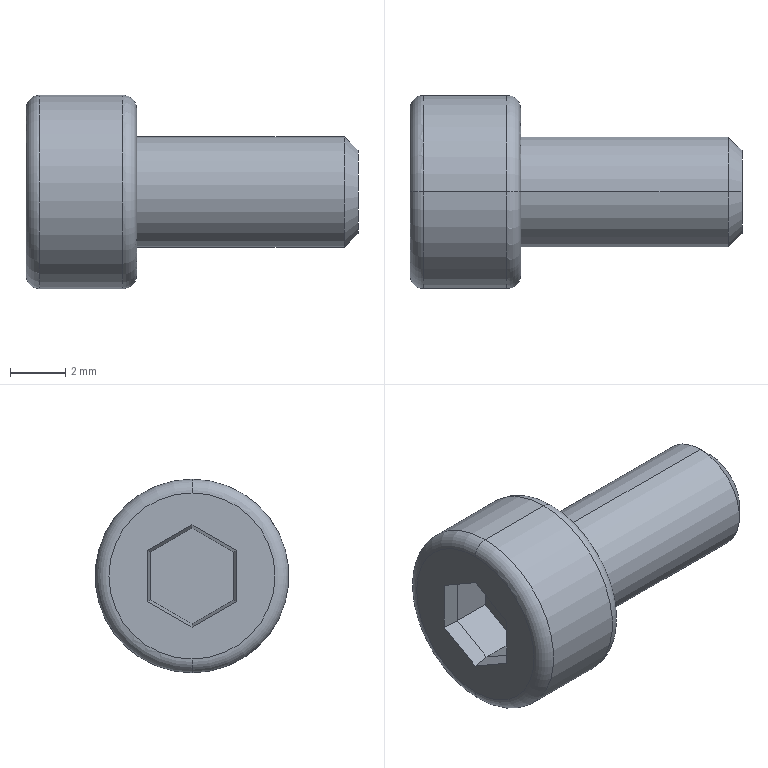Part | SolidWorks | features Chamfer 2, Fillet 1, ICE 1, Revolution 1 | 1 solid | 26 faces | box 12 x 7 x 7 mm | volume 234.855 mm3 | plane 16 | torus 4 | cylinder 4 | cone 2 | commonest cylinder face diameters 4 x2 7 x2
STEP:
#1=CARTESIAN_POINT('',(12.,0.,-1.5));
#2=VERTEX_POINT('',#1);
#3=CARTESIAN_POINT('',(12.,0.,1.5));
#4=VERTEX_POINT('',#3);
#5=CARTESIAN_POINT('',(12.,0.,0.));
#6=DIRECTION('',(1.,0.,0.));
#7=DIRECTION('',(0.,0.,1.));
#8=AXIS2_PLACEMENT_3D('',#5,#6,#7);
#9=CIRCLE('',#8,1.5);
#10=EDGE_CURVE('',#2,#4,#9,.T.);
#11=ORIENTED_EDGE('',*,*,#10,.F.);
#12=CARTESIAN_POINT('',(11.5,0.,-2.));
#13=VERTEX_POINT('',#12);
#14=CARTESIAN_POINT('',(11.5,0.,-2.));
#15=DIRECTION('',(-0.7071,0.,-0.7071));
#16=VECTOR('',#15,1000.);
#17=LINE('',#14,#16);
#18=EDGE_CURVE('',#2,#13,#17,.T.);
#19=ORIENTED_EDGE('',*,*,#18,.T.);
#20=CARTESIAN_POINT('',(11.5,0.,2.));
#21=VERTEX_POINT('',#20);
#22=CARTESIAN_POINT('',(11.5,0.,0.));
#23=DIRECTION('',(-1.,0.,0.));
#24=DIRECTION('',(0.,0.,1.));
#25=AXIS2_PLACEMENT_3D('',#22,#23,#24);
#26=CIRCLE('',#25,2.);
#27=EDGE_CURVE('',#21,#13,#26,.T.);
#28=ORIENTED_EDGE('',*,*,#27,.F.);
#29=CARTESIAN_POINT('',(11.5,0.,2.));
#30=DIRECTION('',(-0.7071,0.,0.7071));
#31=VECTOR('',#30,1000.);
#32=LINE('',#29,#31);
#33=EDGE_CURVE('',#4,#21,#32,.T.);
#34=ORIENTED_EDGE('',*,*,#33,.F.);
#35=EDGE_LOOP('',(#11,#19,#28,#34));
#36=FACE_OUTER_BOUND('',#35,.T.);
#37=CARTESIAN_POINT('',(11.5,0.,0.));
#38=DIRECTION('',(-1.,0.,0.));
#39=DIRECTION('',(0.,0.,1.));
#40=AXIS2_PLACEMENT_3D('',#37,#38,#39);
#41=CONICAL_SURFACE('',#40,2.,0.7854);
#42=ADVANCED_FACE('',(#36),#41,.T.);
#43=CARTESIAN_POINT('',(0.,0.,3.));
#44=VERTEX_POINT('',#43);
#45=CARTESIAN_POINT('',(0.,0.,-3.));
#46=VERTEX_POINT('',#45);
#47=CARTESIAN_POINT('',(0.,0.,0.));
#48=DIRECTION('',(-1.,0.,0.));
#49=DIRECTION('',(0.,0.,-1.));
#50=AXIS2_PLACEMENT_3D('',#47,#48,#49);
#51=CIRCLE('',#50,3.);
#52=EDGE_CURVE('',#44,#46,#51,.T.);
#53=ORIENTED_EDGE('',*,*,#52,.F.);
#54=CARTESIAN_POINT('',(0.5,0.,3.5));
#55=VERTEX_POINT('',#54);
#56=CARTESIAN_POINT('',(0.5,0.,3.));
#57=DIRECTION('',(0.,1.,0.));
#58=DIRECTION('',(0.,0.,1.));
#59=AXIS2_PLACEMENT_3D('',#56,#57,#58);
#60=CIRCLE('',#59,0.5);
#61=EDGE_CURVE('',#44,#55,#60,.T.);
#62=ORIENTED_EDGE('',*,*,#61,.T.);
#63=CARTESIAN_POINT('',(0.5,0.,-3.5));
#64=VERTEX_POINT('',#63);
#65=CARTESIAN_POINT('',(0.5,0.,0.));
#66=DIRECTION('',(1.,0.,0.));
#67=DIRECTION('',(0.,0.,-1.));
#68=AXIS2_PLACEMENT_3D('',#65,#66,#67);
#69=CIRCLE('',#68,3.5);
#70=EDGE_CURVE('',#64,#55,#69,.T.);
#71=ORIENTED_EDGE('',*,*,#70,.F.);
#72=CARTESIAN_POINT('',(0.5,0.,-3.));
#73=DIRECTION('',(0.,-1.,0.));
#74=DIRECTION('',(0.,0.,-1.));
#75=AXIS2_PLACEMENT_3D('',#72,#73,#74);
#76=CIRCLE('',#75,0.5);
#77=EDGE_CURVE('',#46,#64,#76,.T.);
#78=ORIENTED_EDGE('',*,*,#77,.F.);
#79=EDGE_LOOP('',(#53,#62,#71,#78));
#80=FACE_OUTER_BOUND('',#79,.T.);
#81=CARTESIAN_POINT('',(0.5,0.,0.));
#82=DIRECTION('',(1.,0.,0.));
#83=DIRECTION('',(0.,0.,-1.));
#84=AXIS2_PLACEMENT_3D('',#81,#82,#83);
#85=TOROIDAL_SURFACE('',#84,3.,0.5);
#86=ADVANCED_FACE('',(#80),#85,.T.);
#87=CARTESIAN_POINT('',(4.,0.,-3.));
#88=VERTEX_POINT('',#87);
#89=CARTESIAN_POINT('',(4.,0.,3.));
#90=VERTEX_POINT('',#89);
#91=CARTESIAN_POINT('',(4.,0.,0.));
#92=DIRECTION('',(1.,0.,0.));
#93=DIRECTION('',(0.,0.,1.));
#94=AXIS2_PLACEMENT_3D('',#91,#92,#93);
#95=CIRCLE('',#94,3.);
#96=EDGE_CURVE('',#88,#90,#95,.T.);
#97=ORIENTED_EDGE('',*,*,#96,.F.);
#98=CARTESIAN_POINT('',(3.5,0.,-3.5));
#99=VERTEX_POINT('',#98);
#100=CARTESIAN_POINT('',(3.5,0.,-3.));
#101=DIRECTION('',(0.,1.,0.));
#102=DIRECTION('',(0.,0.,1.));
#103=AXIS2_PLACEMENT_3D('',#100,#101,#102);
#104=CIRCLE('',#103,0.5);
#105=EDGE_CURVE('',#88,#99,#104,.T.);
#106=ORIENTED_EDGE('',*,*,#105,.T.);
#107=CARTESIAN_POINT('',(3.5,0.,3.5));
#108=VERTEX_POINT('',#107);
#109=CARTESIAN_POINT('',(3.5,0.,0.));
#110=DIRECTION('',(-1.,0.,0.));
#111=DIRECTION('',(0.,0.,1.));
#112=AXIS2_PLACEMENT_3D('',#109,#110,#111);
#113=CIRCLE('',#112,3.5);
#114=EDGE_CURVE('',#108,#99,#113,.T.);
#115=ORIENTED_EDGE('',*,*,#114,.F.);
#116=CARTESIAN_POINT('',(3.5,0.,3.));
#117=DIRECTION('',(0.,-1.,0.));
#118=DIRECTION('',(0.,0.,-1.));
#119=AXIS2_PLACEMENT_3D('',#116,#117,#118);
#120=CIRCLE('',#119,0.5);
#121=EDGE_CURVE('',#90,#108,#120,.T.);
#122=ORIENTED_EDGE('',*,*,#121,.F.);
#123=EDGE_LOOP('',(#97,#106,#115,#122));
#124=FACE_OUTER_BOUND('',#123,.T.);
#125=CARTESIAN_POINT('',(3.5,0.,0.));
#126=DIRECTION('',(-1.,0.,0.));
#127=DIRECTION('',(0.,0.,1.));
#128=AXIS2_PLACEMENT_3D('',#125,#126,#127);
#129=TOROIDAL_SURFACE('',#128,3.,0.5);
#130=ADVANCED_FACE('',(#124),#129,.T.);
#131=ORIENTED_EDGE('',*,*,#27,.T.);
#132=CARTESIAN_POINT('',(4.,0.,-2.));
#133=VERTEX_POINT('',#132);
#134=CARTESIAN_POINT('',(-4.709,0.,-2.));
#135=DIRECTION('',(-1.,0.,0.));
#136=VECTOR('',#135,1000.);
#137=LINE('',#134,#136);
#138=EDGE_CURVE('',#13,#133,#137,.T.);
#139=ORIENTED_EDGE('',*,*,#138,.T.);
#140=CARTESIAN_POINT('',(4.,0.,2.));
#141=VERTEX_POINT('',#140);
#142=CARTESIAN_POINT('',(4.,0.,0.));
#143=DIRECTION('',(-1.,0.,0.));
#144=DIRECTION('',(0.,0.,1.));
#145=AXIS2_PLACEMENT_3D('',#142,#143,#144);
#146=CIRCLE('',#145,2.);
#147=EDGE_CURVE('',#141,#133,#146,.T.);
#148=ORIENTED_EDGE('',*,*,#147,.F.);
#149=CARTESIAN_POINT('',(-4.709,0.,2.));
#150=DIRECTION('',(-1.,0.,0.));
#151=VECTOR('',#150,1000.);
#152=LINE('',#149,#151);
#153=EDGE_CURVE('',#21,#141,#152,.T.);
#154=ORIENTED_EDGE('',*,*,#153,.F.);
#155=EDGE_LOOP('',(#131,#139,#148,#154));
#156=FACE_OUTER_BOUND('',#155,.T.);
#157=CARTESIAN_POINT('',(-4.709,0.,0.));
#158=DIRECTION('',(-1.,0.,0.));
#159=DIRECTION('',(0.,0.,1.));
#160=AXIS2_PLACEMENT_3D('',#157,#158,#159);
#161=CYLINDRICAL_SURFACE('',#160,2.);
#162=ADVANCED_FACE('',(#156),#161,.T.);
#163=ORIENTED_EDGE('',*,*,#114,.T.);
#164=CARTESIAN_POINT('',(-4.709,0.,-3.5));
#165=DIRECTION('',(-1.,0.,0.));
#166=VECTOR('',#165,1000.);
#167=LINE('',#164,#166);
#168=EDGE_CURVE('',#99,#64,#167,.T.);
#169=ORIENTED_EDGE('',*,*,#168,.T.);
#170=ORIENTED_EDGE('',*,*,#70,.T.);
#171=CARTESIAN_POINT('',(-4.709,0.,3.5));
#172=DIRECTION('',(-1.,0.,0.));
#173=VECTOR('',#172,1000.);
#174=LINE('',#171,#173);
#175=EDGE_CURVE('',#108,#55,#174,.T.);
#176=ORIENTED_EDGE('',*,*,#175,.F.);
#177=EDGE_LOOP('',(#163,#169,#170,#176));
#178=FACE_OUTER_BOUND('',#177,.T.);
#179=CARTESIAN_POINT('',(-4.709,0.,0.));
#180=DIRECTION('',(-1.,0.,0.));
#181=DIRECTION('',(0.,0.,1.));
#182=AXIS2_PLACEMENT_3D('',#179,#180,#181);
#183=CYLINDRICAL_SURFACE('',#182,3.5);
#184=ADVANCED_FACE('',(#178),#183,.T.);
#185=CARTESIAN_POINT('',(0.,-1.6,0.9238));
#186=VERTEX_POINT('',#185);
#187=CARTESIAN_POINT('',(0.,-1.6,-0.9238));
#188=VERTEX_POINT('',#187);
#189=CARTESIAN_POINT('',(0.,-1.6,0.));
#190=DIRECTION('',(0.,0.,-1.));
#191=VECTOR('',#190,1000.);
#192=LINE('',#189,#191);
#193=EDGE_CURVE('',#186,#188,#192,.T.);
#194=ORIENTED_EDGE('',*,*,#193,.T.);
#195=CARTESIAN_POINT('',(0.,0.,-1.848));
#196=VERTEX_POINT('',#195);
#197=CARTESIAN_POINT('',(0.,-0.8,-1.386));
#198=DIRECTION('',(0.,0.866,-0.5));
#199=VECTOR('',#198,1000.);
#200=LINE('',#197,#199);
#201=EDGE_CURVE('',#188,#196,#200,.T.);
#202=ORIENTED_EDGE('',*,*,#201,.T.);
#203=CARTESIAN_POINT('',(0.,1.6,-0.9238));
#204=VERTEX_POINT('',#203);
#205=CARTESIAN_POINT('',(0.,0.8,-1.386));
#206=DIRECTION('',(0.,0.866,0.5));
#207=VECTOR('',#206,1000.);
#208=LINE('',#205,#207);
#209=EDGE_CURVE('',#196,#204,#208,.T.);
#210=ORIENTED_EDGE('',*,*,#209,.T.);
#211=CARTESIAN_POINT('',(0.,1.6,0.9238));
#212=VERTEX_POINT('',#211);
#213=CARTESIAN_POINT('',(0.,1.6,0.));
#214=DIRECTION('',(0.,0.,1.));
#215=VECTOR('',#214,1000.);
#216=LINE('',#213,#215);
#217=EDGE_CURVE('',#204,#212,#216,.T.);
#218=ORIENTED_EDGE('',*,*,#217,.T.);
#219=CARTESIAN_POINT('',(0.,0.,1.848));
#220=VERTEX_POINT('',#219);
#221=CARTESIAN_POINT('',(0.,0.8,1.386));
#222=DIRECTION('',(0.,-0.866,0.5));
#223=VECTOR('',#222,1000.);
#224=LINE('',#221,#223);
#225=EDGE_CURVE('',#212,#220,#224,.T.);
#226=ORIENTED_EDGE('',*,*,#225,.T.);
#227=CARTESIAN_POINT('',(0.,-0.8,1.386));
#228=DIRECTION('',(0.,-0.866,-0.5));
#229=VECTOR('',#228,1000.);
#230=LINE('',#227,#229);
#231=EDGE_CURVE('',#220,#186,#230,.T.);
#232=ORIENTED_EDGE('',*,*,#231,.T.);
#233=EDGE_LOOP('',(#194,#202,#210,#218,#226,#232));
#234=FACE_BOUND('',#233,.T.);
#235=CARTESIAN_POINT('',(0.,0.,0.));
#236=DIRECTION('',(-1.,0.,0.));
#237=DIRECTION('',(0.,0.,-1.));
#238=AXIS2_PLACEMENT_3D('',#235,#236,#237);
#239=CIRCLE('',#238,3.);
#240=EDGE_CURVE('',#46,#44,#239,.T.);
#241=ORIENTED_EDGE('',*,*,#240,.T.);
#242=ORIENTED_EDGE('',*,*,#52,.T.);
#243=EDGE_LOOP('',(#241,#242));
#244=FACE_OUTER_BOUND('',#243,.T.);
#245=CARTESIAN_POINT('',(0.,0.,0.));
#246=DIRECTION('',(1.,0.,0.));
#247=DIRECTION('',(0.,0.,-1.));
#248=AXIS2_PLACEMENT_3D('',#245,#246,#247);
#249=PLANE('',#248);
#250=ADVANCED_FACE('',(#234,#244),#249,.F.);
#251=ORIENTED_EDGE('',*,*,#168,.F.);
#252=CARTESIAN_POINT('',(3.5,0.,0.));
#253=DIRECTION('',(-1.,0.,0.));
#254=DIRECTION('',(0.,0.,1.));
#255=AXIS2_PLACEMENT_3D('',#252,#253,#254);
#256=CIRCLE('',#255,3.5);
#257=EDGE_CURVE('',#99,#108,#256,.T.);
#258=ORIENTED_EDGE('',*,*,#257,.T.);
#259=ORIENTED_EDGE('',*,*,#175,.T.);
#260=CARTESIAN_POINT('',(0.5,0.,0.));
#261=DIRECTION('',(1.,0.,0.));
#262=DIRECTION('',(0.,0.,-1.));
#263=AXIS2_PLACEMENT_3D('',#260,#261,#262);
#264=CIRCLE('',#263,3.5);
#265=EDGE_CURVE('',#55,#64,#264,.T.);
#266=ORIENTED_EDGE('',*,*,#265,.T.);
#267=EDGE_LOOP('',(#251,#258,#259,#266));
#268=FACE_OUTER_BOUND('',#267,.T.);
#269=CARTESIAN_POINT('',(-4.709,0.,0.));
#270=DIRECTION('',(-1.,0.,0.));
#271=DIRECTION('',(0.,0.,1.));
#272=AXIS2_PLACEMENT_3D('',#269,#270,#271);
#273=CYLINDRICAL_SURFACE('',#272,3.5);
#274=ADVANCED_FACE('',(#268),#273,.T.);
#275=CARTESIAN_POINT('',(4.,0.,0.));
#276=DIRECTION('',(1.,0.,0.));
#277=DIRECTION('',(0.,0.,1.));
#278=AXIS2_PLACEMENT_3D('',#275,#276,#277);
#279=CIRCLE('',#278,3.);
#280=EDGE_CURVE('',#90,#88,#279,.T.);
#281=ORIENTED_EDGE('',*,*,#280,.T.);
#282=ORIENTED_EDGE('',*,*,#96,.T.);
#283=EDGE_LOOP('',(#281,#282));
#284=FACE_OUTER_BOUND('',#283,.T.);
#285=ORIENTED_EDGE('',*,*,#147,.T.);
#286=CARTESIAN_POINT('',(4.,0.,0.));
#287=DIRECTION('',(-1.,0.,0.));
#288=DIRECTION('',(0.,0.,1.));
#289=AXIS2_PLACEMENT_3D('',#286,#287,#288);
#290=CIRCLE('',#289,2.);
#291=EDGE_CURVE('',#133,#141,#290,.T.);
#292=ORIENTED_EDGE('',*,*,#291,.T.);
#293=EDGE_LOOP('',(#285,#292));
#294=FACE_BOUND('',#293,.T.);
#295=CARTESIAN_POINT('',(4.,3.5,0.));
#296=DIRECTION('',(-1.,0.,0.));
#297=DIRECTION('',(0.,0.,1.));
#298=AXIS2_PLACEMENT_3D('',#295,#296,#297);
#299=PLANE('',#298);
#300=ADVANCED_FACE('',(#284,#294),#299,.F.);
#301=ORIENTED_EDGE('',*,*,#138,.F.);
#302=CARTESIAN_POINT('',(11.5,0.,0.));
#303=DIRECTION('',(-1.,0.,0.));
#304=DIRECTION('',(0.,0.,1.));
#305=AXIS2_PLACEMENT_3D('',#302,#303,#304);
#306=CIRCLE('',#305,2.);
#307=EDGE_CURVE('',#13,#21,#306,.T.);
#308=ORIENTED_EDGE('',*,*,#307,.T.);
#309=ORIENTED_EDGE('',*,*,#153,.T.);
#310=ORIENTED_EDGE('',*,*,#291,.F.);
#311=EDGE_LOOP('',(#301,#308,#309,#310));
#312=FACE_OUTER_BOUND('',#311,.T.);
#313=CARTESIAN_POINT('',(-4.709,0.,0.));
#314=DIRECTION('',(-1.,0.,0.));
#315=DIRECTION('',(0.,0.,1.));
#316=AXIS2_PLACEMENT_3D('',#313,#314,#315);
#317=CYLINDRICAL_SURFACE('',#316,2.);
#318=ADVANCED_FACE('',(#312),#317,.T.);
#319=CARTESIAN_POINT('',(12.,0.,0.));
#320=DIRECTION('',(1.,0.,0.));
#321=DIRECTION('',(0.,0.,1.));
#322=AXIS2_PLACEMENT_3D('',#319,#320,#321);
#323=CIRCLE('',#322,1.5);
#324=EDGE_CURVE('',#4,#2,#323,.T.);
#325=ORIENTED_EDGE('',*,*,#324,.T.);
#326=ORIENTED_EDGE('',*,*,#10,.T.);
#327=EDGE_LOOP('',(#325,#326));
#328=FACE_OUTER_BOUND('',#327,.T.);
#329=CARTESIAN_POINT('',(12.,2.,0.));
#330=DIRECTION('',(-1.,0.,0.));
#331=DIRECTION('',(0.,0.,1.));
#332=AXIS2_PLACEMENT_3D('',#329,#330,#331);
#333=PLANE('',#332);
#334=ADVANCED_FACE('',(#328),#333,.F.);
#335=CARTESIAN_POINT('',(2.,1.5,-0.866));
#336=VERTEX_POINT('',#335);
#337=CARTESIAN_POINT('',(0.5671,1.5,-0.866));
#338=VERTEX_POINT('',#337);
#339=CARTESIAN_POINT('',(2.,1.5,-0.866));
#340=DIRECTION('',(-1.,0.,0.));
#341=VECTOR('',#340,1000.);
#342=LINE('',#339,#341);
#343=EDGE_CURVE('',#336,#338,#342,.T.);
#344=ORIENTED_EDGE('',*,*,#343,.T.);
#345=CARTESIAN_POINT('',(0.5671,0.,-1.732));
#346=VERTEX_POINT('',#345);
#347=CARTESIAN_POINT('',(0.5671,1.5,-0.866));
#348=DIRECTION('',(0.,-0.866,-0.5));
#349=VECTOR('',#348,1000.);
#350=LINE('',#347,#349);
#351=EDGE_CURVE('',#338,#346,#350,.T.);
#352=ORIENTED_EDGE('',*,*,#351,.T.);
#353=CARTESIAN_POINT('',(2.,0.,-1.732));
#354=VERTEX_POINT('',#353);
#355=CARTESIAN_POINT('',(2.,0.,-1.732));
#356=DIRECTION('',(-1.,0.,0.));
#357=VECTOR('',#356,1000.);
#358=LINE('',#355,#357);
#359=EDGE_CURVE('',#354,#346,#358,.T.);
#360=ORIENTED_EDGE('',*,*,#359,.F.);
#361=CARTESIAN_POINT('',(2.,1.5,-0.866));
#362=DIRECTION('',(0.,-0.866,-0.5));
#363=VECTOR('',#362,1000.);
#364=LINE('',#361,#363);
#365=EDGE_CURVE('',#336,#354,#364,.T.);
#366=ORIENTED_EDGE('',*,*,#365,.F.);
#367=EDGE_LOOP('',(#344,#352,#360,#366));
#368=FACE_OUTER_BOUND('',#367,.T.);
#369=CARTESIAN_POINT('',(2.,1.5,-0.866));
#370=DIRECTION('',(0.,0.5,-0.866));
#371=DIRECTION('',(0.,0.866,0.5));
#372=AXIS2_PLACEMENT_3D('',#369,#370,#371);
#373=PLANE('',#372);
#374=ADVANCED_FACE('',(#368),#373,.F.);
#375=CARTESIAN_POINT('',(2.,1.5,0.866));
#376=VERTEX_POINT('',#375);
#377=CARTESIAN_POINT('',(0.5671,1.5,0.866));
#378=VERTEX_POINT('',#377);
#379=CARTESIAN_POINT('',(2.,1.5,0.866));
#380=DIRECTION('',(-1.,0.,0.));
#381=VECTOR('',#380,1000.);
#382=LINE('',#379,#381);
#383=EDGE_CURVE('',#376,#378,#382,.T.);
#384=ORIENTED_EDGE('',*,*,#383,.T.);
#385=CARTESIAN_POINT('',(0.5671,1.5,0.866));
#386=DIRECTION('',(0.,0.,-1.));
#387=VECTOR('',#386,1000.);
#388=LINE('',#385,#387);
#389=EDGE_CURVE('',#378,#338,#388,.T.);
#390=ORIENTED_EDGE('',*,*,#389,.T.);
#391=ORIENTED_EDGE('',*,*,#343,.F.);
#392=CARTESIAN_POINT('',(2.,1.5,0.866));
#393=DIRECTION('',(0.,0.,-1.));
#394=VECTOR('',#393,1000.);
#395=LINE('',#392,#394);
#396=EDGE_CURVE('',#376,#336,#395,.T.);
#397=ORIENTED_EDGE('',*,*,#396,.F.);
#398=EDGE_LOOP('',(#384,#390,#391,#397));
#399=FACE_OUTER_BOUND('',#398,.T.);
#400=CARTESIAN_POINT('',(2.,1.5,0.866));
#401=DIRECTION('',(0.,1.,0.));
#402=DIRECTION('',(0.,0.,1.));
#403=AXIS2_PLACEMENT_3D('',#400,#401,#402);
#404=PLANE('',#403);
#405=ADVANCED_FACE('',(#399),#404,.F.);
#406=CARTESIAN_POINT('',(2.,0.,1.732));
#407=VERTEX_POINT('',#406);
#408=CARTESIAN_POINT('',(0.5671,0.,1.732));
#409=VERTEX_POINT('',#408);
#410=CARTESIAN_POINT('',(2.,0.,1.732));
#411=DIRECTION('',(-1.,0.,0.));
#412=VECTOR('',#411,1000.);
#413=LINE('',#410,#412);
#414=EDGE_CURVE('',#407,#409,#413,.T.);
#415=ORIENTED_EDGE('',*,*,#414,.T.);
#416=CARTESIAN_POINT('',(0.5671,0.,1.732));
#417=DIRECTION('',(0.,0.866,-0.5));
#418=VECTOR('',#417,1000.);
#419=LINE('',#416,#418);
#420=EDGE_CURVE('',#409,#378,#419,.T.);
#421=ORIENTED_EDGE('',*,*,#420,.T.);
#422=ORIENTED_EDGE('',*,*,#383,.F.);
#423=CARTESIAN_POINT('',(2.,0.,1.732));
#424=DIRECTION('',(0.,0.866,-0.5));
#425=VECTOR('',#424,1000.);
#426=LINE('',#423,#425);
#427=EDGE_CURVE('',#407,#376,#426,.T.);
#428=ORIENTED_EDGE('',*,*,#427,.F.);
#429=EDGE_LOOP('',(#415,#421,#422,#428));
#430=FACE_OUTER_BOUND('',#429,.T.);
#431=CARTESIAN_POINT('',(2.,0.,1.732));
#432=DIRECTION('',(0.,0.5,0.866));
#433=DIRECTION('',(0.,-0.866,0.5));
#434=AXIS2_PLACEMENT_3D('',#431,#432,#433);
#435=PLANE('',#434);
#436=ADVANCED_FACE('',(#430),#435,.F.);
#437=CARTESIAN_POINT('',(2.,-1.5,0.866));
#438=VERTEX_POINT('',#437);
#439=CARTESIAN_POINT('',(0.5671,-1.5,0.866));
#440=VERTEX_POINT('',#439);
#441=CARTESIAN_POINT('',(2.,-1.5,0.866));
#442=DIRECTION('',(-1.,0.,0.));
#443=VECTOR('',#442,1000.);
#444=LINE('',#441,#443);
#445=EDGE_CURVE('',#438,#440,#444,.T.);
#446=ORIENTED_EDGE('',*,*,#445,.T.);
#447=CARTESIAN_POINT('',(0.5671,-1.5,0.866));
#448=DIRECTION('',(0.,0.866,0.5));
#449=VECTOR('',#448,1000.);
#450=LINE('',#447,#449);
#451=EDGE_CURVE('',#440,#409,#450,.T.);
#452=ORIENTED_EDGE('',*,*,#451,.T.);
#453=ORIENTED_EDGE('',*,*,#414,.F.);
#454=CARTESIAN_POINT('',(2.,-1.5,0.866));
#455=DIRECTION('',(0.,0.866,0.5));
#456=VECTOR('',#455,1000.);
#457=LINE('',#454,#456);
#458=EDGE_CURVE('',#438,#407,#457,.T.);
#459=ORIENTED_EDGE('',*,*,#458,.F.);
#460=EDGE_LOOP('',(#446,#452,#453,#459));
#461=FACE_OUTER_BOUND('',#460,.T.);
#462=CARTESIAN_POINT('',(2.,-1.5,0.866));
#463=DIRECTION('',(0.,-0.5,0.866));
#464=DIRECTION('',(0.,-0.866,-0.5));
#465=AXIS2_PLACEMENT_3D('',#462,#463,#464);
#466=PLANE('',#465);
#467=ADVANCED_FACE('',(#461),#466,.F.);
#468=CARTESIAN_POINT('',(2.,-1.5,-0.866));
#469=VERTEX_POINT('',#468);
#470=CARTESIAN_POINT('',(0.5671,-1.5,-0.866));
#471=VERTEX_POINT('',#470);
#472=CARTESIAN_POINT('',(2.,-1.5,-0.866));
#473=DIRECTION('',(-1.,0.,0.));
#474=VECTOR('',#473,1000.);
#475=LINE('',#472,#474);
#476=EDGE_CURVE('',#469,#471,#475,.T.);
#477=ORIENTED_EDGE('',*,*,#476,.T.);
#478=CARTESIAN_POINT('',(0.5671,-1.5,-0.866));
#479=DIRECTION('',(0.,0.,1.));
#480=VECTOR('',#479,1000.);
#481=LINE('',#478,#480);
#482=EDGE_CURVE('',#471,#440,#481,.T.);
#483=ORIENTED_EDGE('',*,*,#482,.T.);
#484=ORIENTED_EDGE('',*,*,#445,.F.);
#485=CARTESIAN_POINT('',(2.,-1.5,-0.866));
#486=DIRECTION('',(0.,0.,1.));
#487=VECTOR('',#486,1000.);
#488=LINE('',#485,#487);
#489=EDGE_CURVE('',#469,#438,#488,.T.);
#490=ORIENTED_EDGE('',*,*,#489,.F.);
#491=EDGE_LOOP('',(#477,#483,#484,#490));
#492=FACE_OUTER_BOUND('',#491,.T.);
#493=CARTESIAN_POINT('',(2.,-1.5,-0.866));
#494=DIRECTION('',(0.,-1.,0.));
#495=DIRECTION('',(0.,0.,-1.));
#496=AXIS2_PLACEMENT_3D('',#493,#494,#495);
#497=PLANE('',#496);
#498=ADVANCED_FACE('',(#492),#497,.F.);
#499=ORIENTED_EDGE('',*,*,#359,.T.);
#500=CARTESIAN_POINT('',(0.5671,0.,-1.732));
#501=DIRECTION('',(0.,-0.866,0.5));
#502=VECTOR('',#501,1000.);
#503=LINE('',#500,#502);
#504=EDGE_CURVE('',#346,#471,#503,.T.);
#505=ORIENTED_EDGE('',*,*,#504,.T.);
#506=ORIENTED_EDGE('',*,*,#476,.F.);
#507=CARTESIAN_POINT('',(2.,0.,-1.732));
#508=DIRECTION('',(0.,-0.866,0.5));
#509=VECTOR('',#508,1000.);
#510=LINE('',#507,#509);
#511=EDGE_CURVE('',#354,#469,#510,.T.);
#512=ORIENTED_EDGE('',*,*,#511,.F.);
#513=EDGE_LOOP('',(#499,#505,#506,#512));
#514=FACE_OUTER_BOUND('',#513,.T.);
#515=CARTESIAN_POINT('',(2.,0.,-1.732));
#516=DIRECTION('',(0.,-0.5,-0.866));
#517=DIRECTION('',(0.,0.866,-0.5));
#518=AXIS2_PLACEMENT_3D('',#515,#516,#517);
#519=PLANE('',#518);
#520=ADVANCED_FACE('',(#514),#519,.F.);
#521=ORIENTED_EDGE('',*,*,#365,.T.);
#522=ORIENTED_EDGE('',*,*,#511,.T.);
#523=ORIENTED_EDGE('',*,*,#489,.T.);
#524=ORIENTED_EDGE('',*,*,#458,.T.);
#525=ORIENTED_EDGE('',*,*,#427,.T.);
#526=ORIENTED_EDGE('',*,*,#396,.T.);
#527=EDGE_LOOP('',(#521,#522,#523,#524,#525,#526));
#528=FACE_OUTER_BOUND('',#527,.T.);
#529=CARTESIAN_POINT('',(2.,0.,0.));
#530=DIRECTION('',(-1.,0.,0.));
#531=DIRECTION('',(0.,0.,1.));
#532=AXIS2_PLACEMENT_3D('',#529,#530,#531);
#533=PLANE('',#532);
#534=ADVANCED_FACE('',(#528),#533,.T.);
#535=ORIENTED_EDGE('',*,*,#105,.F.);
#536=ORIENTED_EDGE('',*,*,#280,.F.);
#537=ORIENTED_EDGE('',*,*,#121,.T.);
#538=ORIENTED_EDGE('',*,*,#257,.F.);
#539=EDGE_LOOP('',(#535,#536,#537,#538));
#540=FACE_OUTER_BOUND('',#539,.T.);
#541=CARTESIAN_POINT('',(3.5,0.,0.));
#542=DIRECTION('',(-1.,0.,0.));
#543=DIRECTION('',(0.,0.,1.));
#544=AXIS2_PLACEMENT_3D('',#541,#542,#543);
#545=TOROIDAL_SURFACE('',#544,3.,0.5);
#546=ADVANCED_FACE('',(#540),#545,.T.);
#547=ORIENTED_EDGE('',*,*,#61,.F.);
#548=ORIENTED_EDGE('',*,*,#240,.F.);
#549=ORIENTED_EDGE('',*,*,#77,.T.);
#550=ORIENTED_EDGE('',*,*,#265,.F.);
#551=EDGE_LOOP('',(#547,#548,#549,#550));
#552=FACE_OUTER_BOUND('',#551,.T.);
#553=CARTESIAN_POINT('',(0.5,0.,0.));
#554=DIRECTION('',(1.,0.,0.));
#555=DIRECTION('',(0.,0.,-1.));
#556=AXIS2_PLACEMENT_3D('',#553,#554,#555);
#557=TOROIDAL_SURFACE('',#556,3.,0.5);
#558=ADVANCED_FACE('',(#552),#557,.T.);
#559=CARTESIAN_POINT('',(0.7364,0.,1.698));
#560=DIRECTION('',(0.9799,0.,-0.1995));
#561=VECTOR('',#560,1000.);
#562=LINE('',#559,#561);
#563=EDGE_CURVE('',#220,#409,#562,.T.);
#564=ORIENTED_EDGE('',*,*,#563,.F.);
#565=ORIENTED_EDGE('',*,*,#225,.F.);
#566=CARTESIAN_POINT('',(0.7364,1.47,0.8488));
#567=DIRECTION('',(-0.9799,0.1728,0.09976));
#568=VECTOR('',#567,1000.);
#569=LINE('',#566,#568);
#570=EDGE_CURVE('',#378,#212,#569,.T.);
#571=ORIENTED_EDGE('',*,*,#570,.F.);
#572=ORIENTED_EDGE('',*,*,#420,.F.);
#573=EDGE_LOOP('',(#564,#565,#571,#572));
#574=FACE_OUTER_BOUND('',#573,.T.);
#575=CARTESIAN_POINT('',(0.5671,0.,1.732));
#576=DIRECTION('',(0.1736,0.4924,0.8529));
#577=DIRECTION('',(0.,0.866,-0.5));
#578=AXIS2_PLACEMENT_3D('',#575,#576,#577);
#579=PLANE('',#578);
#580=ADVANCED_FACE('',(#574),#579,.F.);
#581=ORIENTED_EDGE('',*,*,#570,.T.);
#582=ORIENTED_EDGE('',*,*,#217,.F.);
#583=CARTESIAN_POINT('',(0.7364,1.47,-0.8488));
#584=DIRECTION('',(-0.9799,0.1728,-0.09976));
#585=VECTOR('',#584,1000.);
#586=LINE('',#583,#585);
#587=EDGE_CURVE('',#338,#204,#586,.T.);
#588=ORIENTED_EDGE('',*,*,#587,.F.);
#589=ORIENTED_EDGE('',*,*,#389,.F.);
#590=EDGE_LOOP('',(#581,#582,#588,#589));
#591=FACE_OUTER_BOUND('',#590,.T.);
#592=CARTESIAN_POINT('',(0.5671,1.5,0.866));
#593=DIRECTION('',(0.1736,0.9848,0.));
#594=DIRECTION('',(0.,0.,-1.));
#595=AXIS2_PLACEMENT_3D('',#592,#593,#594);
#596=PLANE('',#595);
#597=ADVANCED_FACE('',(#591),#596,.F.);
#598=ORIENTED_EDGE('',*,*,#563,.T.);
#599=ORIENTED_EDGE('',*,*,#451,.F.);
#600=CARTESIAN_POINT('',(0.7364,-1.47,0.8488));
#601=DIRECTION('',(0.9799,0.1728,-0.09976));
#602=VECTOR('',#601,1000.);
#603=LINE('',#600,#602);
#604=EDGE_CURVE('',#186,#440,#603,.T.);
#605=ORIENTED_EDGE('',*,*,#604,.F.);
#606=ORIENTED_EDGE('',*,*,#231,.F.);
#607=EDGE_LOOP('',(#598,#599,#605,#606));
#608=FACE_OUTER_BOUND('',#607,.T.);
#609=CARTESIAN_POINT('',(0.5671,-1.5,0.866));
#610=DIRECTION('',(0.1736,-0.4924,0.8529));
#611=DIRECTION('',(0.,0.866,0.5));
#612=AXIS2_PLACEMENT_3D('',#609,#610,#611);
#613=PLANE('',#612);
#614=ADVANCED_FACE('',(#608),#613,.F.);
#615=ORIENTED_EDGE('',*,*,#587,.T.);
#616=ORIENTED_EDGE('',*,*,#209,.F.);
#617=CARTESIAN_POINT('',(0.5671,0.,-1.732));
#618=DIRECTION('',(-0.9799,0.,-0.1995));
#619=VECTOR('',#618,1000.);
#620=LINE('',#617,#619);
#621=EDGE_CURVE('',#346,#196,#620,.T.);
#622=ORIENTED_EDGE('',*,*,#621,.F.);
#623=ORIENTED_EDGE('',*,*,#351,.F.);
#624=EDGE_LOOP('',(#615,#616,#622,#623));
#625=FACE_OUTER_BOUND('',#624,.T.);
#626=CARTESIAN_POINT('',(0.5671,1.5,-0.866));
#627=DIRECTION('',(0.1736,0.4924,-0.8529));
#628=DIRECTION('',(0.,-0.866,-0.5));
#629=AXIS2_PLACEMENT_3D('',#626,#627,#628);
#630=PLANE('',#629);
#631=ADVANCED_FACE('',(#625),#630,.F.);
#632=ORIENTED_EDGE('',*,*,#604,.T.);
#633=ORIENTED_EDGE('',*,*,#482,.F.);
#634=CARTESIAN_POINT('',(0.7364,-1.47,-0.8488));
#635=DIRECTION('',(0.9799,0.1728,0.09976));
#636=VECTOR('',#635,1000.);
#637=LINE('',#634,#636);
#638=EDGE_CURVE('',#188,#471,#637,.T.);
#639=ORIENTED_EDGE('',*,*,#638,.F.);
#640=ORIENTED_EDGE('',*,*,#193,.F.);
#641=EDGE_LOOP('',(#632,#633,#639,#640));
#642=FACE_OUTER_BOUND('',#641,.T.);
#643=CARTESIAN_POINT('',(0.5671,-1.5,-0.866));
#644=DIRECTION('',(0.1736,-0.9848,0.));
#645=DIRECTION('',(0.,0.,1.));
#646=AXIS2_PLACEMENT_3D('',#643,#644,#645);
#647=PLANE('',#646);
#648=ADVANCED_FACE('',(#642),#647,.F.);
#649=ORIENTED_EDGE('',*,*,#621,.T.);
#650=ORIENTED_EDGE('',*,*,#201,.F.);
#651=ORIENTED_EDGE('',*,*,#638,.T.);
#652=ORIENTED_EDGE('',*,*,#504,.F.);
#653=EDGE_LOOP('',(#649,#650,#651,#652));
#654=FACE_OUTER_BOUND('',#653,.T.);
#655=CARTESIAN_POINT('',(0.5671,0.,-1.732));
#656=DIRECTION('',(0.1736,-0.4924,-0.8529));
#657=DIRECTION('',(0.,-0.866,0.5));
#658=AXIS2_PLACEMENT_3D('',#655,#656,#657);
#659=PLANE('',#658);
#660=ADVANCED_FACE('',(#654),#659,.F.);
#661=ORIENTED_EDGE('',*,*,#18,.F.);
#662=ORIENTED_EDGE('',*,*,#324,.F.);
#663=ORIENTED_EDGE('',*,*,#33,.T.);
#664=ORIENTED_EDGE('',*,*,#307,.F.);
#665=EDGE_LOOP('',(#661,#662,#663,#664));
#666=FACE_OUTER_BOUND('',#665,.T.);
#667=CARTESIAN_POINT('',(11.5,0.,0.));
#668=DIRECTION('',(-1.,0.,0.));
#669=DIRECTION('',(0.,0.,1.));
#670=AXIS2_PLACEMENT_3D('',#667,#668,#669);
#671=CONICAL_SURFACE('',#670,2.,0.7854);
#672=ADVANCED_FACE('',(#666),#671,.T.);
#673=CLOSED_SHELL('',(#42,#86,#130,#162,#184,#250,#274,#300,#318,#334,#374,#405,#436,#467,#498,#520,#534,#546,#558,#580,#597,#614,#631,#648,#660,#672));
#674=MANIFOLD_SOLID_BREP('',#673);
#675=CARTESIAN_POINT('',(0.,0.,0.));
#676=DIRECTION('',(0.,0.,1.));
#677=DIRECTION('',(1.,0.,0.));
#678=AXIS2_PLACEMENT_3D('',#675,#676,#677);
#679=(LENGTH_UNIT()NAMED_UNIT(*)SI_UNIT(.MILLI.,.METRE.));
#680=UNCERTAINTY_MEASURE_WITH_UNIT(LENGTH_MEASURE(0.00001),#679,'','');
#681=(NAMED_UNIT(*)PLANE_ANGLE_UNIT()SI_UNIT($,.RADIAN.));
#682=(NAMED_UNIT(*)SI_UNIT($,.STERADIAN.)SOLID_ANGLE_UNIT());
#683=(GEOMETRIC_REPRESENTATION_CONTEXT(3)GLOBAL_UNCERTAINTY_ASSIGNED_CONTEXT((#680))GLOBAL_UNIT_ASSIGNED_CONTEXT((#679,#681,#682))REPRESENTATION_CONTEXT('',''));
#684=ADVANCED_BREP_SHAPE_REPRESENTATION('',(#674,#678),#683);